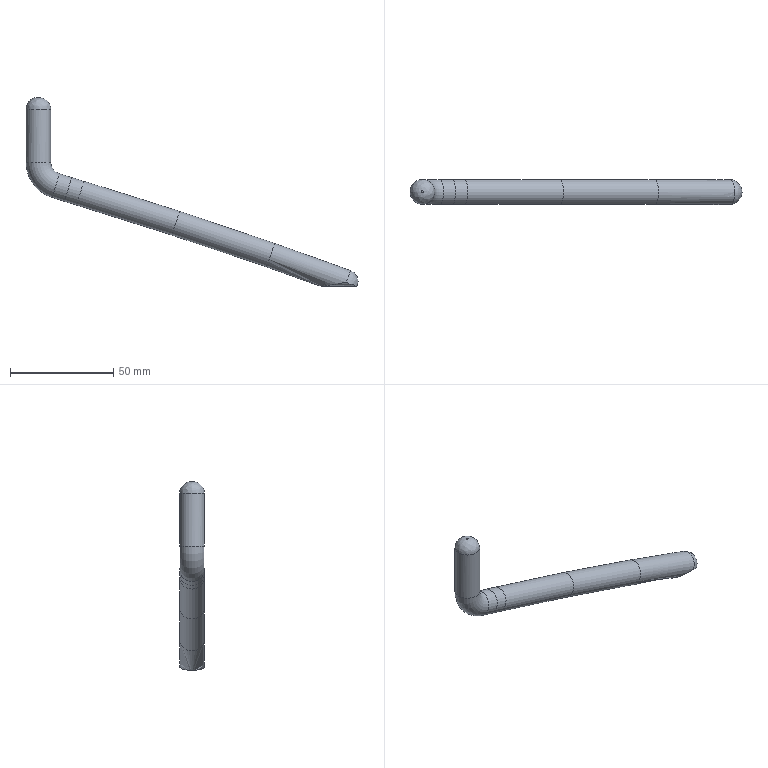Part | STEP file | solid 25 | 1 solid | 14 faces | box 160.634 x 12 x 91.227 mm | volume 21883 mm3 | torus 6 | spline 3 | other 3 | plane 2